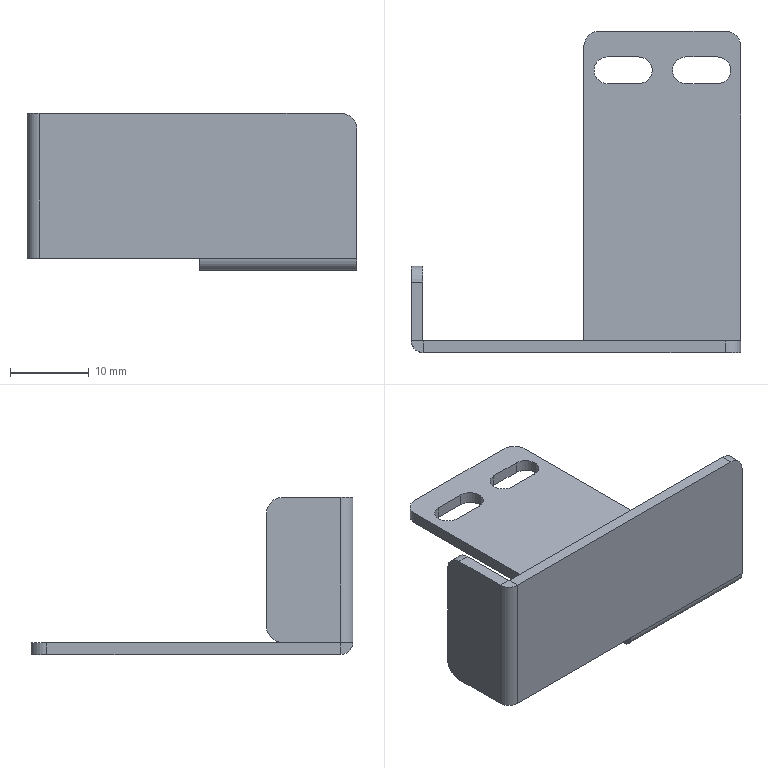Part | STEP file | 1 solid | 38 faces | box 42 x 41 x 20 mm | volume 2562 mm3 | plane 23 | cylinder 15 | commonest cylinder face diameters 3.4 x6 4 x5 0.1 x2 3.1 x2